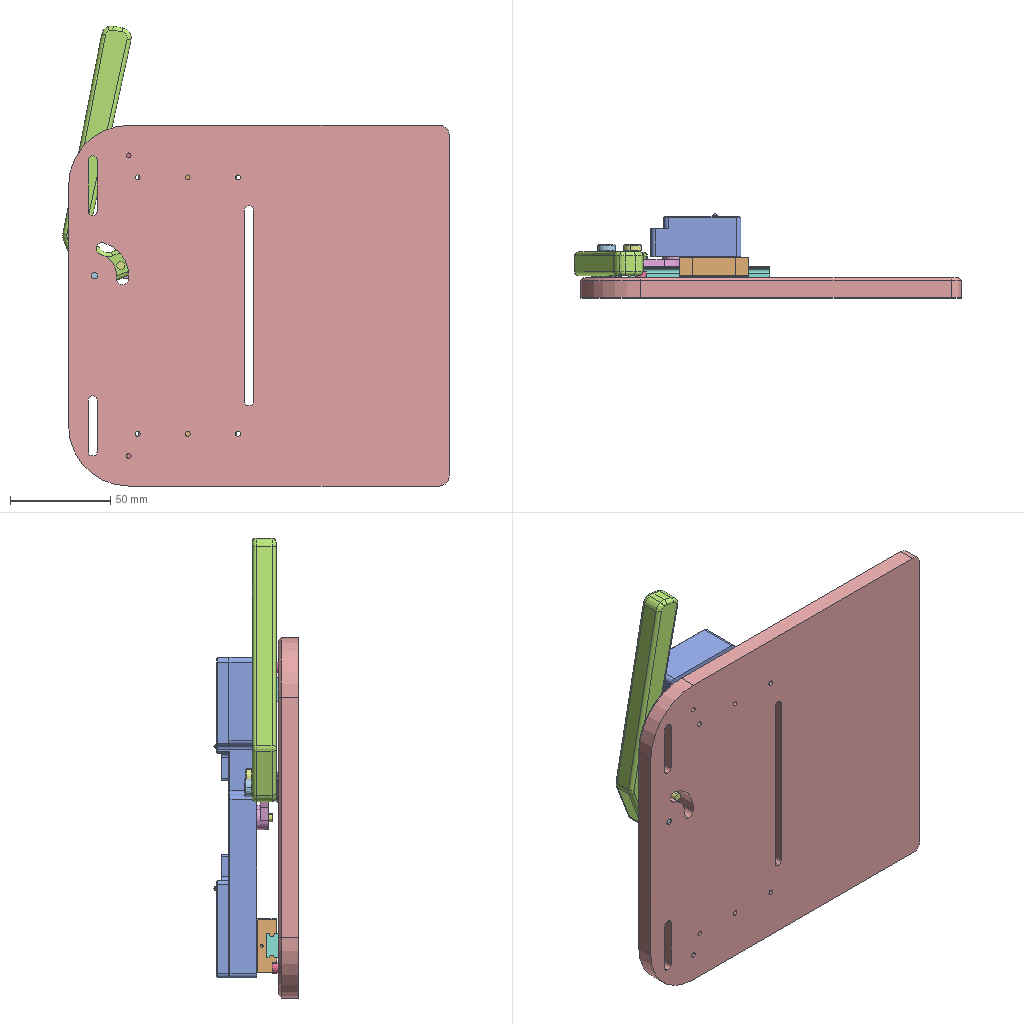Assembly | SolidWorks | 16 different items | 22 placed | box 193 x 42 x 230 mm
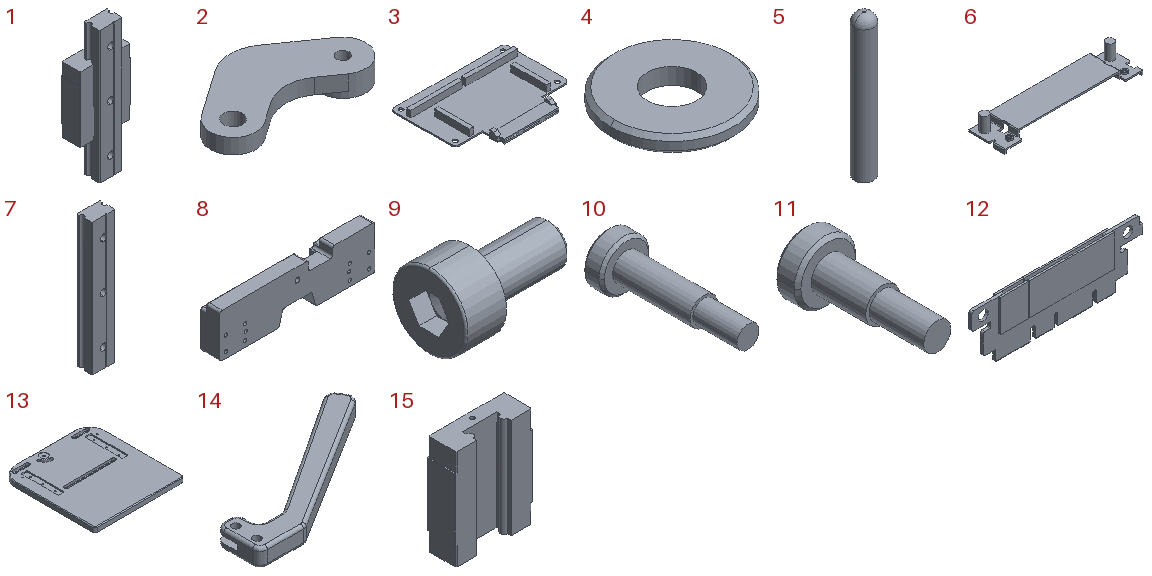Parts list (item | name | quantity | parent item | size | volume | features):
1 | (subassembly) | x2 | - | 27 x 13 x 70 mm | 12887 mm3 | -
2 | - | x1 | - | 41 x 21.27 x 5.6 mm | 2205 mm3 | features Attribute 3, ICE 2, Extrusion 1, Fillet 1, HoleWzd 1
3 | - | x1 | - | 141 x 103.9 x 11.65 mm | 34757 mm3 | features ICE 6, Attribute 3, Chamfer 1, Extrusion 1, Fillet 1
4 | - | x1 | - | 15 x 15 x 2 mm | 285.361 mm3 | features Attribute 3, Chamfer 1, Extrusion 1
5 | - | x2 | - | 2.2 x 2.2 x 16 mm | 59.639 mm3 | features Attribute 3, Extrusion 1, Fillet 1
6 | - | x1 | - | 93.1 x 23.2 x 12.8 mm | 2476 mm3 | features ICE 7, Attribute 3, Extrusion 1, Fillet 1
7 | - | x2 | in 1 | 12 x 8 x 70 mm | 5872 mm3 | features Attribute 3, BaseBody 1
8 | - | x1 | - | 160 x 20 x 45 mm | 104785 mm3 | features Cut 7, ICE 3, Fillet 2, HoleWzd 2, Chamfer 1, Extrusion 1
9 | - | x2 | - | 9 x 5.5 x 5.5 mm | 104.631 mm3 | features Fillet 2, RevCut 2, Cut 1, LPattern 1, Revolution 1
10 | - | x1 | - | 9 x 25.5 x 9 mm | 575.685 mm3 | features Attribute 3, Chamfer 1, ICE 1, Revolution 1
11 | - | x2 | - | 9 x 19.5 x 9 mm | 457.876 mm3 | features Attribute 3, Chamfer 1, ICE 1, Revolution 1
12 | - | x1 | - | 90.5 x 3.57 x 29.5 mm | 4915 mm3 | features BaseBody 1, ICE 1, Split 1
13 | - | x1 | - | 180 x 190 x 10 mm | 321054 mm3 | features HoleWzd 4, Attribute 3, Cut 3, Fillet 3, Chamfer 1, Extrusion 1, ICE 1, LPattern 1
14 | - | x1 | - | 119.634 x 67.923 x 11.9 mm | 22865 mm3 | features ICE 5, Attribute 3, Fillet 2, Extrusion 1
15 | - | x2 | in 1 | 27 x 10 x 34.7 mm | 7015 mm3 | features Attribute 3, BaseBody 1
16 | Wave Solder Hold-Down Clip | x1 | - | - | - | -
Mates (type | each side: item.copy, entity, surface, feature):
In the top assembly
Coincident | 12.1 face plane Input1 | 6.1 face plane Boss-Extrude1
Width | 6.1 face plane Boss-Extrude2 | 6.1 face plane Boss-Extrude2 | 12.1 face plane Input1 | 12.1 face plane Input1
Coincident | 12.1 face plane Input1 | 6.1 face plane Cut-Extrude4
Coincident | 8.1 face plane Cut-Extrude1 | 12.1 face plane Input1 | 2 times
Width | 6.1 face plane Boss-Extrude1 | 6.1 face plane Boss-Extrude1 | 8.1 face plane Cut-Extrude1 | 8.1 face plane Cut-Extrude1
Coincident | 13.1 face plane Boss-Extrude1 | assembly plane | 3 times
Width | 12.1 face plane Input1 | 12.1 face plane Input1 | 3.1 face plane Cut-Extrude2 | 3.1 face plane Cut-Extrude2
Width | 12.1 face plane Input1 | 12.1 face plane Input1 | 3.1 face plane Boss-Extrude2 | 3.1 face plane Boss-Extrude2
LimitDistanceDim | 12.1 face plane Input1 | 3.1 face plane Cut-Extrude3
DistanceDim | 7.1 face plane Input1 | 13.1 face plane Cut-Extrude1
Width | 7.1 face plane Input1 | 7.1 face plane Input1 | 13.1 face plane Cut-Extrude1 | 13.1 face plane Cut-Extrude1
Concentric | 13.1 face cylinder Cut-Extrude2 | 14.1 face cylinder Cut-Extrude2
Concentric | 14.1 face cylinder Cut-Extrude2 | 2.1 face cylinder Cut-Extrude1
Coincident | 14.1 face plane Cut-Extrude3 | 2.1 face plane Boss-Extrude1
Concentric | 8.1 face cylinder Cut-Extrude19 | 2.1 face cylinder M4 Tapped Hole1
Concentric | 13.1 face cylinder M3 Tapped Hole2 | 9.1 face cylinder Base-Revolve
Coincident | 13.1 face plane Boss-Extrude1 | 9.1 face plane Base-Revolve
Concentric | 13.1 face cylinder M3 Tapped Hole2 | 9.2 face cylinder Base-Revolve
Coincident | 13.1 face plane Boss-Extrude1 | 9.2 face plane Base-Revolve
Coincident | 8.1 face plane Boss-Extrude1 | 15.1 face plane Input1
Coincident | 8.1 face plane Cut-Extrude18 | 5.1 face plane Boss-Extrude1
Concentric | 8.1 face cylinder Cut-Extrude18 | 5.1 face cylinder Boss-Extrude1
Coincident | 8.1 face plane Cut-Extrude18 | 5.2 face plane Boss-Extrude1
Concentric | 8.1 face cylinder Cut-Extrude18 | 5.2 face cylinder Boss-Extrude1
Coincident | 13.1 face plane Cut-Extrude4 | 4.1 face plane Boss-Extrude1
Concentric | 13.1 face cylinder Cut-Extrude4 | 4.1 face cylinder Boss-Extrude1
DistanceDim | 13.1 face plane Boss-Extrude1 | 14.1 face plane Boss-Extrude1
Concentric | 8.1 face cylinder Cut-Extrude20 | 11.1 face cylinder Revolve1
Coincident | 2.1 face plane Boss-Extrude2 | 11.1 face plane Revolve1
Coincident | 13.1 face plane Cut-Extrude4 | 10.1 face plane Revolve1
Concentric | 14.1 face cylinder Cut-Extrude2 | 10.1 face cylinder Revolve1
Concentric | 14.1 face cylinder Cut-Extrude4 | 11.2 face cylinder Revolve1
Coincident | 14.1 face plane Cut-Extrude3 | 11.2 face plane Revolve1
In subassembly 1
Concentric | 7.2 face cylinder Input1 | 15.2 face cylinder Input1 | 2 times
LimitDistanceDim | 15.2 face plane Input1 | 7.2 face plane Input1